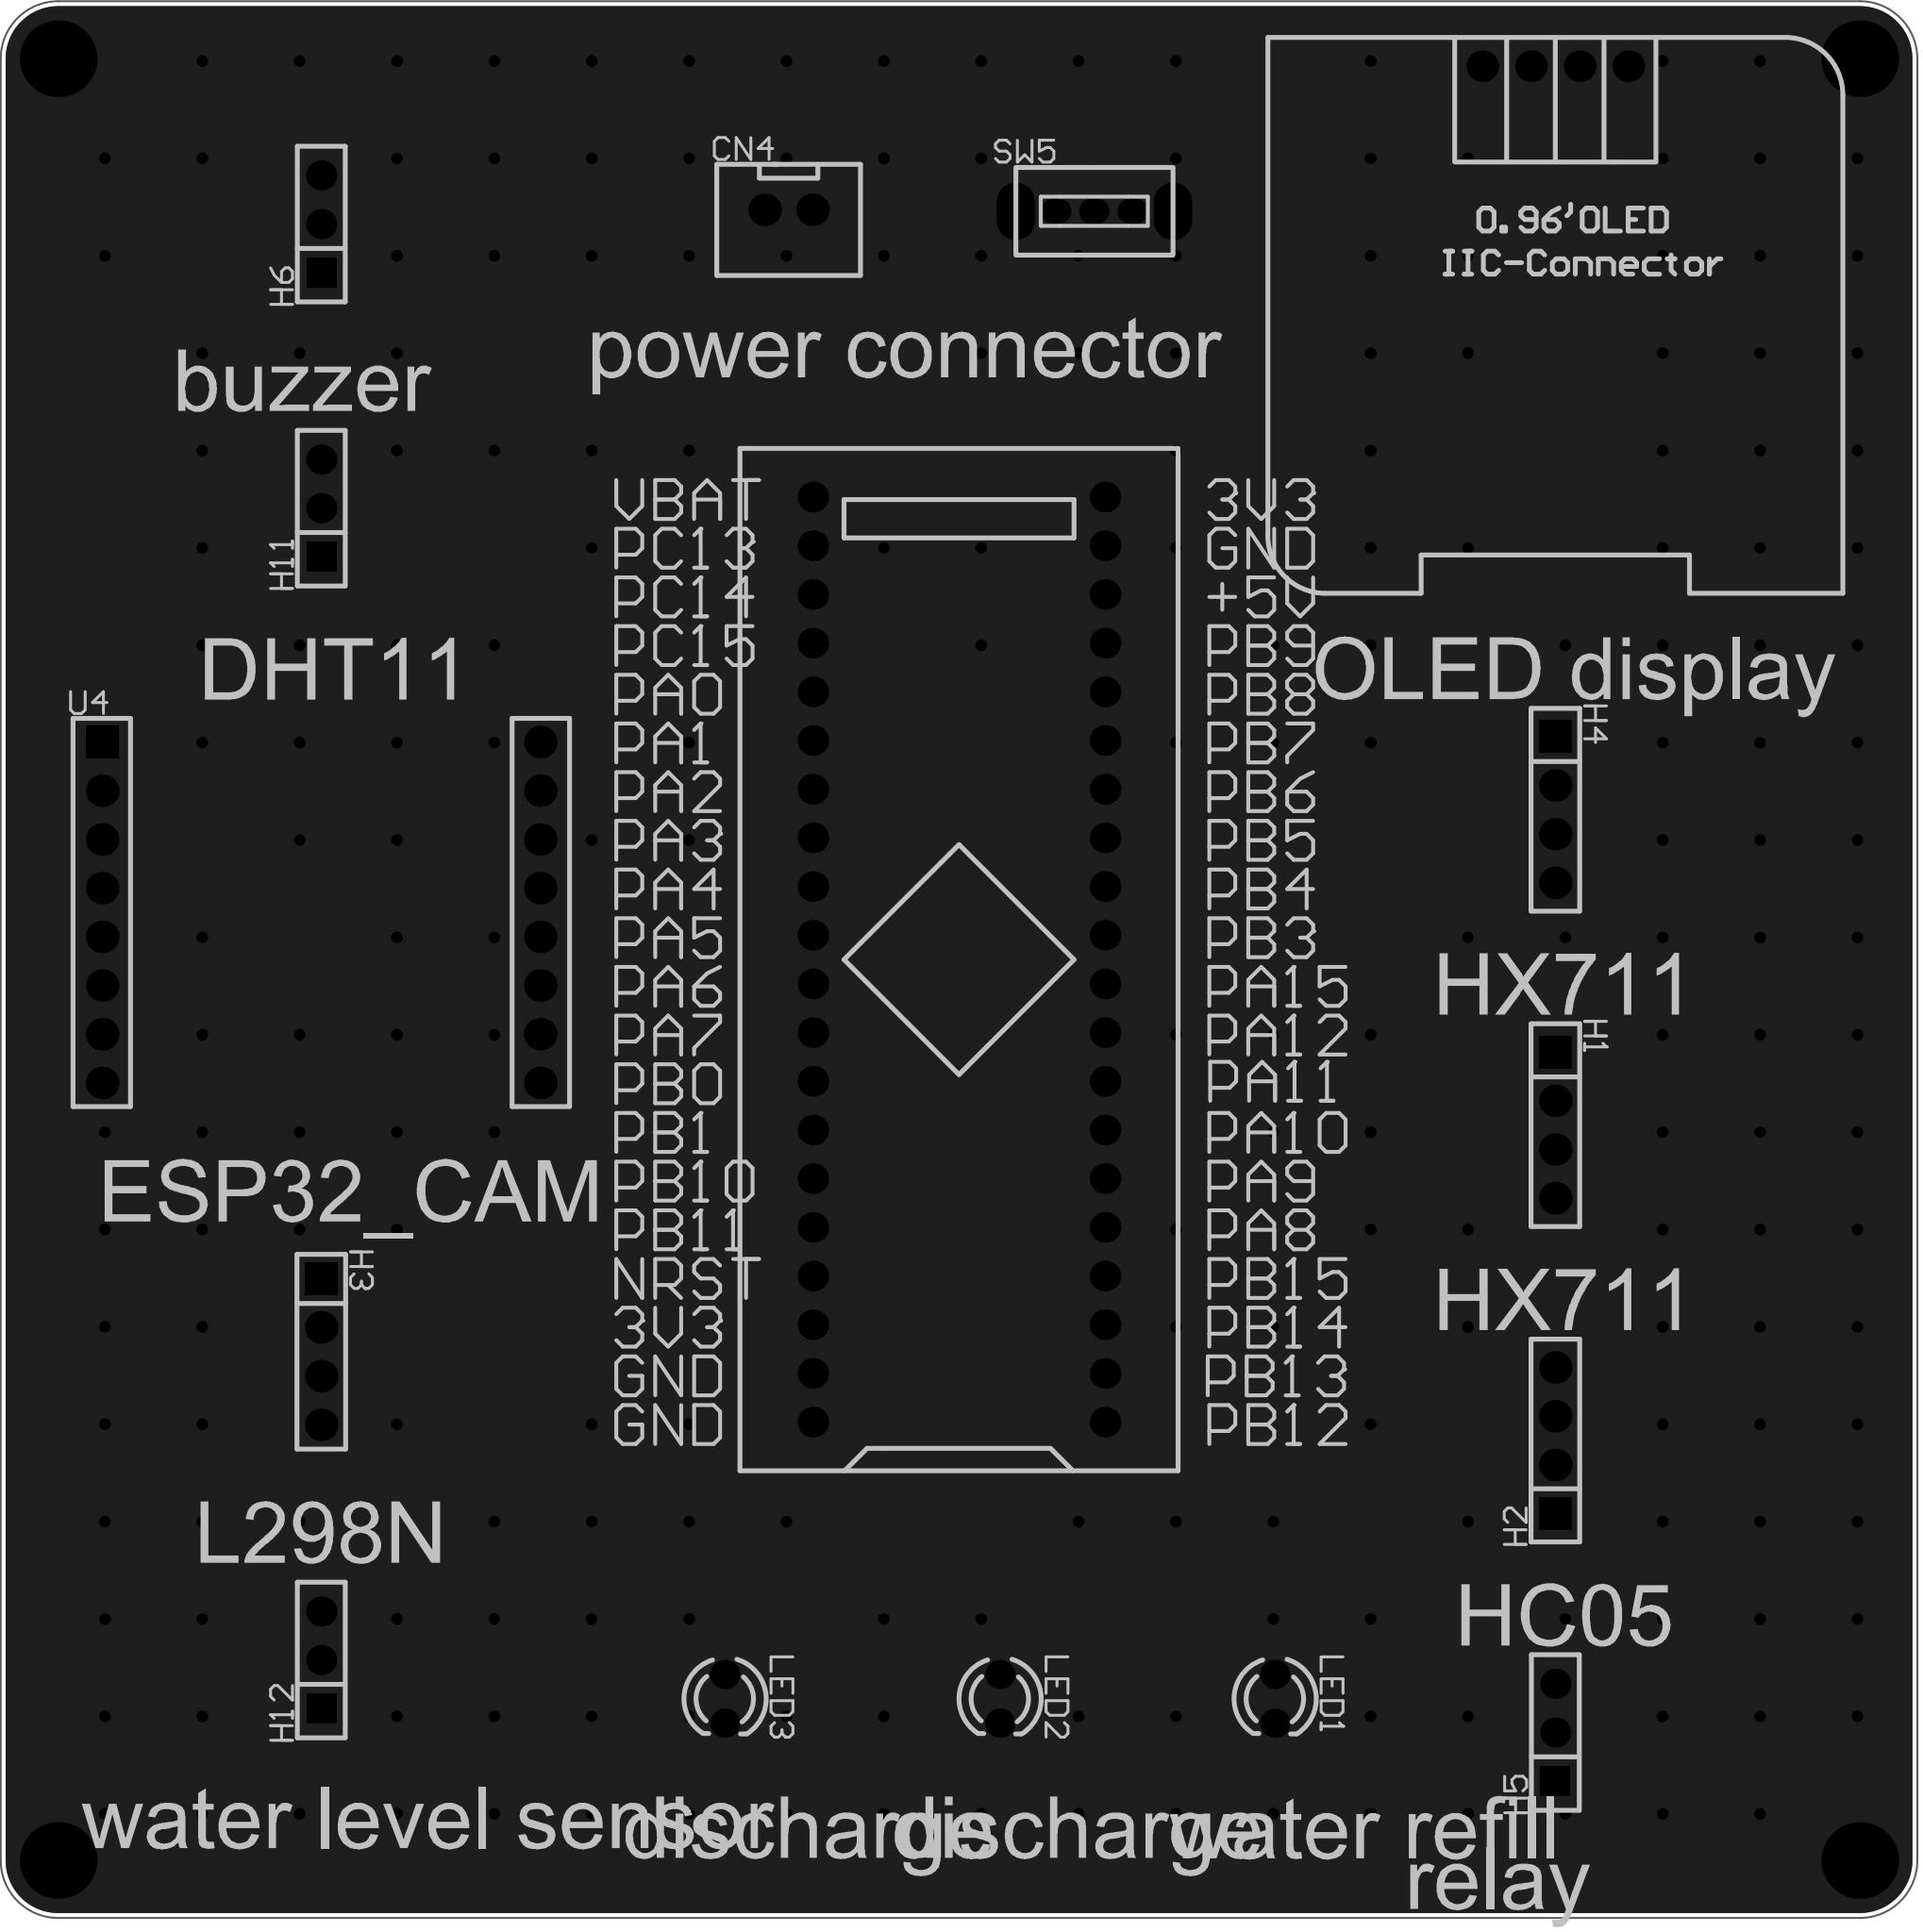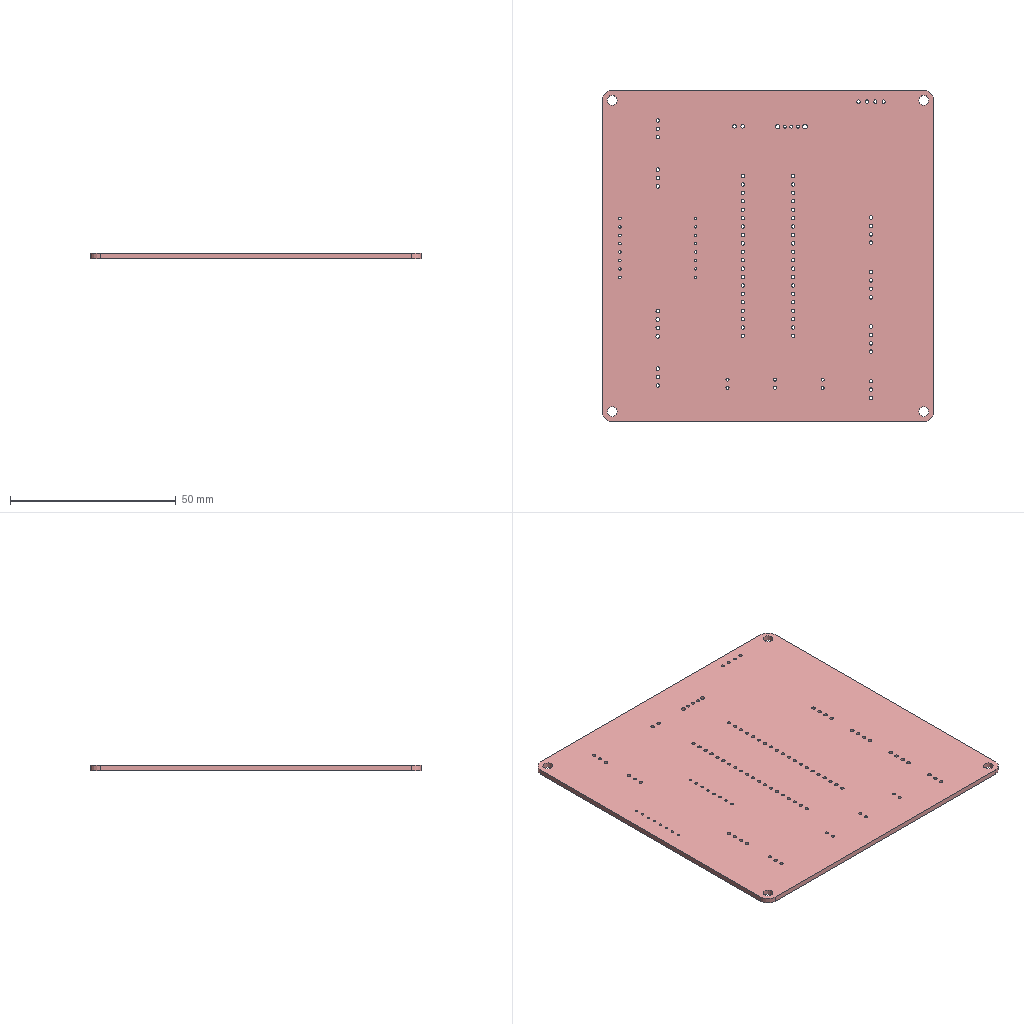Circuit board layout | Altium Designer | box 100 x 100 x 1.6 mm
Layer stack:
# Altium Designer layer stack of  (unit mm; dielectric type: 0 none, 1 core, 2 prepreg, 3 surface material)
index,name,kind,layer,copper_thickness_mm,dielectric_type,dielectric_thickness_mm,dielectric_material,dielectric_constant
0,Top Paste Mask Layer,other,,,,,,
1,Top Silkscreen Layer,other,,,,,,
2,Top Solder Mask Layer,dielectric,,,3,0.01,,3.3
3,Top Layer,copper,Top Layer,0.035,,,,
4,Dielectric1,dielectric,,,3,1.51,FR4,4.5
5,Bottom Layer,copper,Bottom Layer,0.035,,,,
6,Bottom Solder Mask Layer,dielectric,,,3,0.01,,3.3
7,Bottom Silkscreen Layer,other,,,,,,
8,Bottom Paste Mask Layer,other,,,,,,
# drill layer pairs: low layer,high layer
drill_pair,Top Layer,Bottom Layer
Part placement:
Designator,Comment,Layer,Footprint,Center-X(mm),Center-Y(mm),Rotation
U1,STM32F103C8T6-Card,TopLayer,CONN-TH_L53.3-W22.9_STM32F103C8T6-CARD,141.351,130.937,90
OLED1,,TopLayer,0.96OLED_4P,172.466,177.546,0
H11,,TopLayer,HDR-TH_3P-P2.54-V-F,108.077,154.488,90
H12,,TopLayer,HDR-TH_3P-P2.54-V-F,108.077,94.394,90
CN4,XH2.54*2P_through-hole,TopLayer,CONN-TH_2P-P2.50-XH2.54-2P,132.461,170.053,0
SW5,,TopLayer,拨动开关,148.417,169.978,0
H1,,TopLayer,HDR-TH_4P-P2.54-V-F,172.466,122.299,270
H2,,TopLayer,HDR-TH_4P-P2.54-V-F,172.466,105.845,90
H3,,TopLayer,HDR-TH_4P-P2.54-V-M,108.077,110.478,270
H4,,TopLayer,HDR-TH_4P-P2.54-V-F,172.466,138.754,270
H5,,TopLayer,HDR-TH_3P-P2.54-V-F,172.466,90.613,90
H6,,TopLayer,HDR-TH_3P-P2.54-V-F,108.077,169.31,90
LED1,,TopLayer,LED_TH-3mm,157.831,92.368,270
LED2,,TopLayer,LED_TH-3mm,143.48,92.368,270
LED3,,TopLayer,LED_TH-3mm,129.129,92.368,270
U4,ESP32_CAM,TopLayer,ESP32-CAM,108.077,133.395,0
Pad and via stacks:
# Altium Designer via and pad stacks of  (unit mm). Each distinct definition once, with the count of objects using it.
# via: kind,start_layer,end_layer,hole_mm,diameter_mm,mode(0 simple;1 top-mid-bottom;2 full stack),diameter_per_layer,count,example_net
# pad: kind,layer,hole_mm,hole_type(0 round;1 square;2 slot),plating,top_size,top_shape(1 round;2 rect;3 octagon;9 rounded rect),mid_size,bottom_size,mode,footprint,size_per_layer,count,example
pad,Multi-Layer,3,0,plated,4x4,1,4x4,4x4,0,,,4,1
pad,Multi-Layer,1,0,plated,1.6x1.6,1,1.6x1.6,1.6x1.6,0,CONN-TH_L53.3-W22.9_STM32F103C8T6-CARD,,40,U1.1
pad,Multi-Layer,1,0,plated,1.65x1.65,1,1.65x1.65,1.65x1.65,0,0.96OLED_4P,,4,OLED1.4
pad,Multi-Layer,1.02,0,plated,1.575x1.575,1,1.575x1.575,1.575x1.575,0,HDR-TH_3P-P2.54-V-F,,8,H11.3
pad,Multi-Layer,1.02,0,plated,1.575x1.575,2,1.575x1.575,1.575x1.575,0,HDR-TH_3P-P2.54-V-F,,4,H11.1
pad,Multi-Layer,1.05,0,plated,1.7x1.7,1,1.7x1.7,1.7x1.7,0,CONN-TH_2P-P2.50-XH2.54-2P,,2,CN4.2
pad,Multi-Layer,0.8992,0,plated,1.6x1.3,1,1.6x1.3,1.6x1.3,0,\u00B2\u00A6\u00B6\u00AF\u00BF\u00AA\u00B9\u00D8,,3,SW5.1
pad,Multi-Layer,1.3,0,plated,3x1.999,1,3x1.999,3x1.999,0,\u00B2\u00A6\u00B6\u00AF\u00BF\u00AA\u00B9\u00D8,,2,SW5.4
pad,Multi-Layer,1.1,0,plated,1.7x1.7,2,1.7x1.7,1.7x1.7,0,HDR-TH_4P-P2.54-V-F,,3,H1.1
pad,Multi-Layer,1.1,0,plated,1.7x1.7,1,1.7x1.7,1.7x1.7,0,HDR-TH_4P-P2.54-V-F,,9,H1.2
pad,Multi-Layer,1.1,0,plated,1.7x1.7,2,1.7x1.7,1.7x1.7,0,HDR-TH_4P-P2.54-V-M,,1,H3.1
pad,Multi-Layer,1.1,0,plated,1.7x1.7,1,1.7x1.7,1.7x1.7,0,HDR-TH_4P-P2.54-V-M,,3,H3.2
pad,Multi-Layer,0.9144,0,plated,1.524x1.524,1,1.524x1.524,1.524x1.524,0,LED_TH-3mm,,6,LED1.1
pad,Multi-Layer,0.75,0,plated,1.7x1.7,1,1.7x1.7,1.7x1.7,0,ESP32-CAM,,15,U4.16
pad,Multi-Layer,0.75,0,plated,1.7x1.7,2,1.7x1.7,1.7x1.7,0,ESP32-CAM,,1,U4.1
via,Top Layer,Bottom Layer,0.3048,0.61,0,,220,GND
Copper pours:
name,layer,net,type(0 solid;1 hatched;2 none)
Bottom Layer-GND,Bottom Layer,GND,0
Top Layer-GND,Top Layer,GND,0